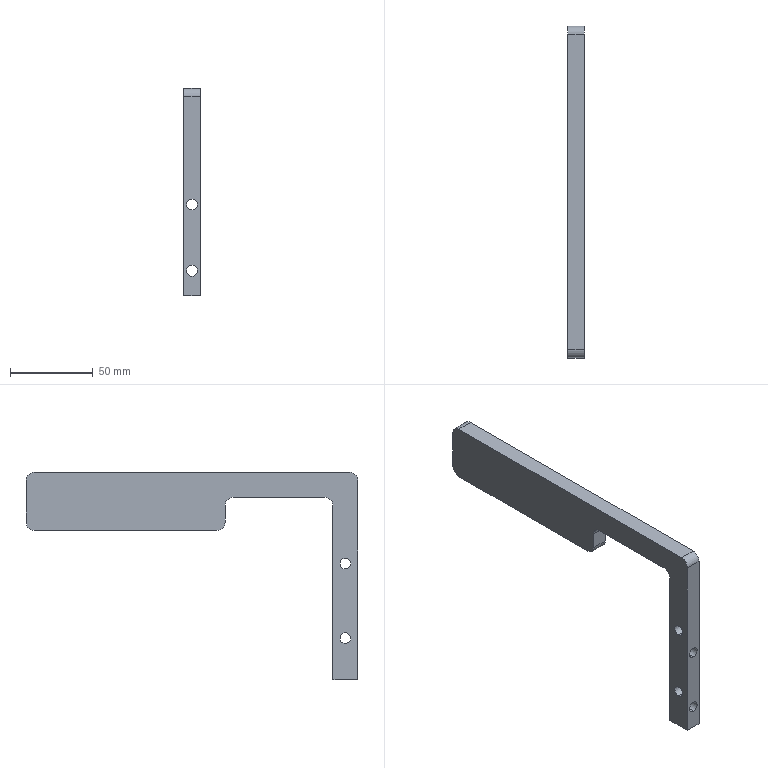Part | STEP file | PN_0019 | 1 solid | 36 faces | box 10 x 200 x 125 mm | volume 67703 mm3 | cylinder 20 | plane 10 | cone 6 | commonest cylinder face diameters 6.5 x8 5 x6 10 x6